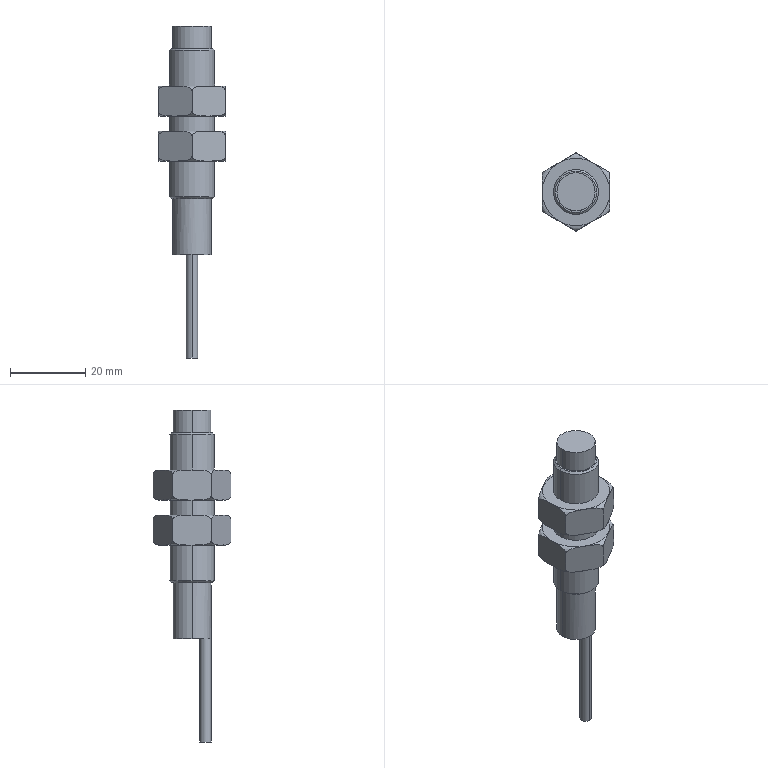Part | STEP file | 001-004-TE-12N4C, _TE-12N4C | 1 solid | 61 faces | box 18 x 20.785 x 88.5 mm | volume 9092 mm3 | torus 24 | plane 21 | cylinder 12 | cone 4 | commonest cylinder face diameters 12 x6 10.2 x4 3 x2